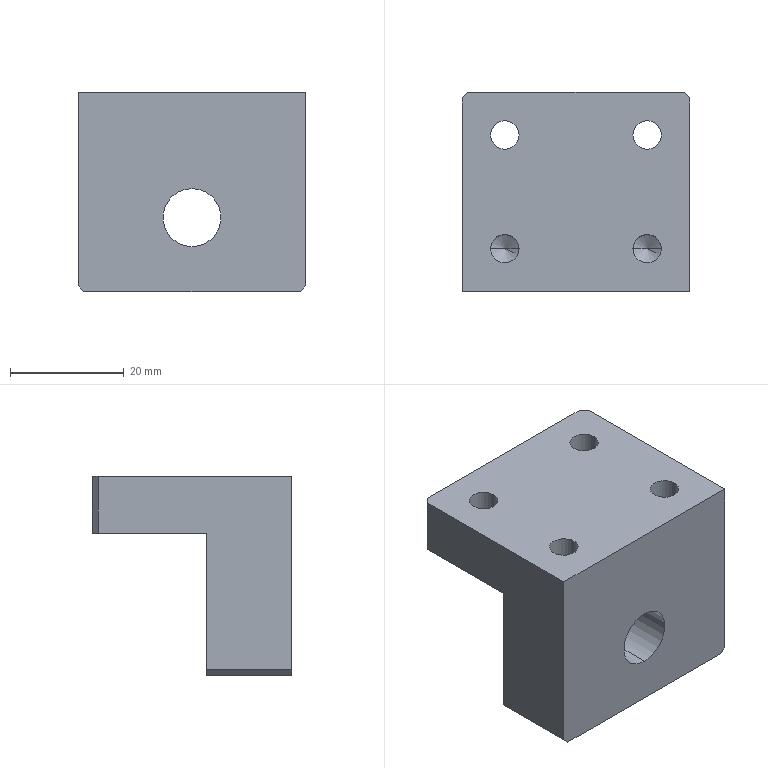Part | STEP file | Fixing block 2 | 1 solid | 32 faces | box 40 x 35 x 35 mm | volume 25797 mm3 | cylinder 14 | plane 14 | cone 4 | commonest cylinder face diameters 5 x8 3.3 x2 6 x2 10.2 x2